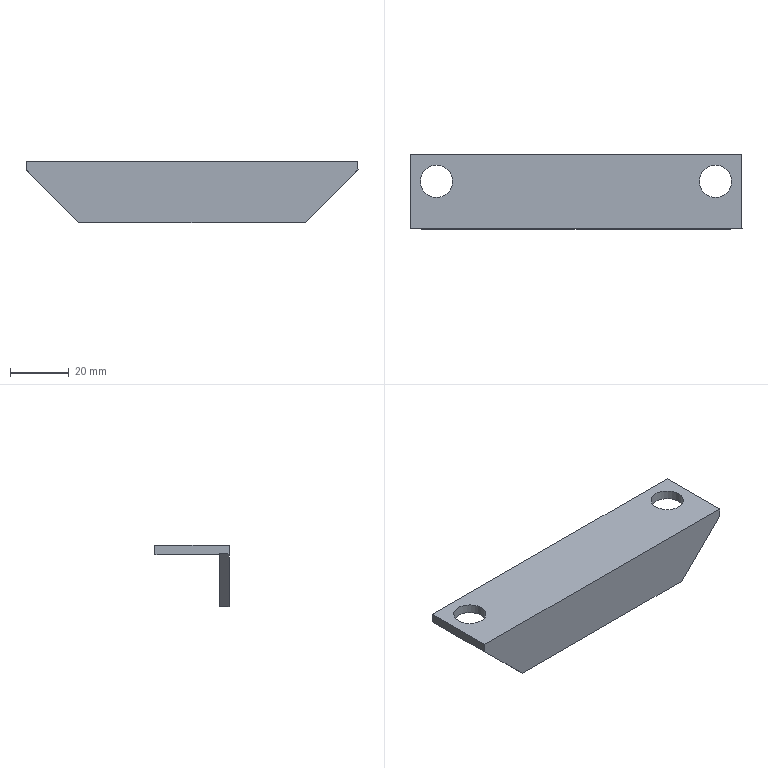Part | NX | features solid 2 | 1 solid | 14 faces | box 113 x 25.2 x 21 mm | volume 13904 mm3 | plane 12 | cylinder 2 | commonest cylinder face diameters 11 x2
STEP:
#1=CARTESIAN_POINT('',(-352.8,-53.5,401.8));
#2=VERTEX_POINT('',#1);
#3=CARTESIAN_POINT('',(-240.2,-53.5,401.8));
#4=VERTEX_POINT('',#3);
#5=CARTESIAN_POINT('',(-353.,-53.5,401.8));
#6=DIRECTION('',(1.,0.000000011,0.000000001));
#7=VECTOR('',#6,1000.);
#8=LINE('',#5,#7);
#9=EDGE_CURVE('',#2,#4,#8,.T.);
#10=ORIENTED_EDGE('',*,*,#9,.T.);
#11=CARTESIAN_POINT('',(-258.,-53.5,384.));
#12=VERTEX_POINT('',#11);
#13=CARTESIAN_POINT('',(-258.,-53.5,384.));
#14=DIRECTION('',(-0.7071,-0.000000128,-0.7071));
#15=VECTOR('',#14,1000.);
#16=LINE('',#13,#15);
#17=EDGE_CURVE('',#12,#4,#16,.F.);
#18=ORIENTED_EDGE('',*,*,#17,.F.);
#19=CARTESIAN_POINT('',(-335.,-53.5,384.));
#20=VERTEX_POINT('',#19);
#21=CARTESIAN_POINT('',(-353.,-53.5,384.));
#22=DIRECTION('',(1.,0.000000011,0.000000001));
#23=VECTOR('',#22,1000.);
#24=LINE('',#21,#23);
#25=EDGE_CURVE('',#20,#12,#24,.T.);
#26=ORIENTED_EDGE('',*,*,#25,.F.);
#27=CARTESIAN_POINT('',(-353.,-53.5,402.));
#28=DIRECTION('',(0.7071,-0.000000113,-0.7071));
#29=VECTOR('',#28,1000.);
#30=LINE('',#27,#29);
#31=EDGE_CURVE('',#2,#20,#30,.T.);
#32=ORIENTED_EDGE('',*,*,#31,.F.);
#33=EDGE_LOOP('',(#10,#18,#26,#32));
#34=FACE_BOUND('',#33,.T.);
#35=CARTESIAN_POINT('',(-353.,-53.5,379.));
#36=DIRECTION('',(0.000000011,-1.,0.00000017));
#37=DIRECTION('',(0.000000001,-0.00000017,-1.));
#38=AXIS2_PLACEMENT_3D('',#35,#36,#37);
#39=PLANE('',#38);
#40=ADVANCED_FACE('',(#34),#39,.F.);
#41=CARTESIAN_POINT('',(-353.,-56.7,405.));
#42=VERTEX_POINT('',#41);
#43=CARTESIAN_POINT('',(-240.,-56.7,405.));
#44=VERTEX_POINT('',#43);
#45=CARTESIAN_POINT('',(-353.,-56.7,405.));
#46=DIRECTION('',(1.,0.000000011,0.000000001));
#47=VECTOR('',#46,1000.);
#48=LINE('',#45,#47);
#49=EDGE_CURVE('',#42,#44,#48,.T.);
#50=ORIENTED_EDGE('',*,*,#49,.T.);
#51=CARTESIAN_POINT('',(-240.,-31.5,405.));
#52=VERTEX_POINT('',#51);
#53=CARTESIAN_POINT('',(-240.,-53.5,405.));
#54=DIRECTION('',(0.000000011,-1.,0.00000017));
#55=VECTOR('',#54,1000.);
#56=LINE('',#53,#55);
#57=EDGE_CURVE('',#52,#44,#56,.T.);
#58=ORIENTED_EDGE('',*,*,#57,.F.);
#59=CARTESIAN_POINT('',(-353.,-31.5,405.));
#60=VERTEX_POINT('',#59);
#61=CARTESIAN_POINT('',(-353.,-31.5,405.));
#62=DIRECTION('',(1.,0.000000011,0.000000001));
#63=VECTOR('',#62,1000.);
#64=LINE('',#61,#63);
#65=EDGE_CURVE('',#60,#52,#64,.T.);
#66=ORIENTED_EDGE('',*,*,#65,.F.);
#67=CARTESIAN_POINT('',(-353.,-53.5,405.));
#68=DIRECTION('',(0.000000011,-1.,0.00000017));
#69=VECTOR('',#68,1000.);
#70=LINE('',#67,#69);
#71=EDGE_CURVE('',#60,#42,#70,.T.);
#72=ORIENTED_EDGE('',*,*,#71,.T.);
#73=EDGE_LOOP('',(#50,#58,#66,#72));
#74=FACE_BOUND('',#73,.T.);
#75=CARTESIAN_POINT('',(-254.5,-40.5,405.));
#76=VERTEX_POINT('',#75);
#77=CARTESIAN_POINT('',(-249.,-40.5,405.));
#78=DIRECTION('',(-0.000000001,0.00000017,1.));
#79=DIRECTION('',(-1.,-0.000000011,-0.000000001));
#80=AXIS2_PLACEMENT_3D('',#77,#78,#79);
#81=CIRCLE('',#80,5.5);
#82=EDGE_CURVE('',#76,#76,#81,.F.);
#83=ORIENTED_EDGE('',*,*,#82,.T.);
#84=EDGE_LOOP('',(#83));
#85=FACE_BOUND('',#84,.T.);
#86=CARTESIAN_POINT('',(-349.5,-40.5,405.));
#87=VERTEX_POINT('',#86);
#88=CARTESIAN_POINT('',(-344.,-40.5,405.));
#89=DIRECTION('',(-0.000000001,0.00000017,1.));
#90=DIRECTION('',(-1.,-0.000000011,-0.000000001));
#91=AXIS2_PLACEMENT_3D('',#88,#89,#90);
#92=CIRCLE('',#91,5.5);
#93=EDGE_CURVE('',#87,#87,#92,.F.);
#94=ORIENTED_EDGE('',*,*,#93,.T.);
#95=EDGE_LOOP('',(#94));
#96=FACE_BOUND('',#95,.T.);
#97=CARTESIAN_POINT('',(-353.,-53.5,405.));
#98=DIRECTION('',(0.000000001,-0.00000017,-1.));
#99=DIRECTION('',(1.,0.000000011,0.000000001));
#100=AXIS2_PLACEMENT_3D('',#97,#98,#99);
#101=PLANE('',#100);
#102=ADVANCED_FACE('',(#74,#85,#96),#101,.F.);
#103=ORIENTED_EDGE('',*,*,#71,.F.);
#104=CARTESIAN_POINT('',(-353.,-31.5,401.8));
#105=VERTEX_POINT('',#104);
#106=CARTESIAN_POINT('',(-353.,-31.5,405.));
#107=DIRECTION('',(0.000000001,-0.00000017,-1.));
#108=VECTOR('',#107,1000.);
#109=LINE('',#106,#108);
#110=EDGE_CURVE('',#60,#105,#109,.T.);
#111=ORIENTED_EDGE('',*,*,#110,.T.);
#112=CARTESIAN_POINT('',(-353.,-53.5,401.8));
#113=VERTEX_POINT('',#112);
#114=CARTESIAN_POINT('',(-353.,-56.7,401.8));
#115=DIRECTION('',(0.000000011,-1.,0.00000017));
#116=VECTOR('',#115,1000.);
#117=LINE('',#114,#116);
#118=EDGE_CURVE('',#105,#113,#117,.T.);
#119=ORIENTED_EDGE('',*,*,#118,.T.);
#120=CARTESIAN_POINT('',(-353.,-53.5,402.));
#121=VERTEX_POINT('',#120);
#122=CARTESIAN_POINT('',(-353.,-53.5,405.));
#123=DIRECTION('',(0.000000001,-0.00000017,-1.));
#124=VECTOR('',#123,1000.);
#125=LINE('',#122,#124);
#126=EDGE_CURVE('',#121,#113,#125,.T.);
#127=ORIENTED_EDGE('',*,*,#126,.F.);
#128=CARTESIAN_POINT('',(-353.,-56.7,402.));
#129=VERTEX_POINT('',#128);
#130=CARTESIAN_POINT('',(-353.,-53.5,402.));
#131=DIRECTION('',(-0.000000011,1.,-0.00000017));
#132=VECTOR('',#131,1000.);
#133=LINE('',#130,#132);
#134=EDGE_CURVE('',#129,#121,#133,.T.);
#135=ORIENTED_EDGE('',*,*,#134,.F.);
#136=CARTESIAN_POINT('',(-353.,-56.7,405.));
#137=DIRECTION('',(0.000000001,-0.00000017,-1.));
#138=VECTOR('',#137,1000.);
#139=LINE('',#136,#138);
#140=EDGE_CURVE('',#42,#129,#139,.T.);
#141=ORIENTED_EDGE('',*,*,#140,.F.);
#142=EDGE_LOOP('',(#103,#111,#119,#127,#135,#141));
#143=FACE_BOUND('',#142,.T.);
#144=CARTESIAN_POINT('',(-353.,-53.5,405.));
#145=DIRECTION('',(-1.,-0.000000011,-0.000000001));
#146=DIRECTION('',(0.000000001,-0.00000017,-1.));
#147=AXIS2_PLACEMENT_3D('',#144,#145,#146);
#148=PLANE('',#147);
#149=ADVANCED_FACE('',(#143),#148,.T.);
#150=CARTESIAN_POINT('',(-240.,-56.7,402.));
#151=VERTEX_POINT('',#150);
#152=CARTESIAN_POINT('',(-240.,-56.7,405.));
#153=DIRECTION('',(0.000000001,-0.00000017,-1.));
#154=VECTOR('',#153,1000.);
#155=LINE('',#152,#154);
#156=EDGE_CURVE('',#44,#151,#155,.T.);
#157=ORIENTED_EDGE('',*,*,#156,.T.);
#158=CARTESIAN_POINT('',(-240.,-53.5,402.));
#159=VERTEX_POINT('',#158);
#160=CARTESIAN_POINT('',(-240.,-53.5,402.));
#161=DIRECTION('',(0.000000011,-1.,0.00000017));
#162=VECTOR('',#161,1000.);
#163=LINE('',#160,#162);
#164=EDGE_CURVE('',#159,#151,#163,.T.);
#165=ORIENTED_EDGE('',*,*,#164,.F.);
#166=CARTESIAN_POINT('',(-240.,-53.5,401.8));
#167=VERTEX_POINT('',#166);
#168=CARTESIAN_POINT('',(-240.,-53.5,405.));
#169=DIRECTION('',(0.000000001,-0.00000017,-1.));
#170=VECTOR('',#169,1000.);
#171=LINE('',#168,#170);
#172=EDGE_CURVE('',#159,#167,#171,.T.);
#173=ORIENTED_EDGE('',*,*,#172,.T.);
#174=CARTESIAN_POINT('',(-240.,-31.5,401.8));
#175=VERTEX_POINT('',#174);
#176=CARTESIAN_POINT('',(-240.,-56.7,401.8));
#177=DIRECTION('',(0.000000011,-1.,0.00000017));
#178=VECTOR('',#177,1000.);
#179=LINE('',#176,#178);
#180=EDGE_CURVE('',#175,#167,#179,.T.);
#181=ORIENTED_EDGE('',*,*,#180,.F.);
#182=CARTESIAN_POINT('',(-240.,-31.5,405.));
#183=DIRECTION('',(0.000000001,-0.00000017,-1.));
#184=VECTOR('',#183,1000.);
#185=LINE('',#182,#184);
#186=EDGE_CURVE('',#52,#175,#185,.T.);
#187=ORIENTED_EDGE('',*,*,#186,.F.);
#188=ORIENTED_EDGE('',*,*,#57,.T.);
#189=EDGE_LOOP('',(#157,#165,#173,#181,#187,#188));
#190=FACE_BOUND('',#189,.T.);
#191=CARTESIAN_POINT('',(-240.,-53.5,405.));
#192=DIRECTION('',(-1.,-0.000000011,-0.000000001));
#193=DIRECTION('',(0.000000001,-0.00000017,-1.));
#194=AXIS2_PLACEMENT_3D('',#191,#192,#193);
#195=PLANE('',#194);
#196=ADVANCED_FACE('',(#190),#195,.F.);
#197=CARTESIAN_POINT('',(-335.,-56.7,384.));
#198=VERTEX_POINT('',#197);
#199=CARTESIAN_POINT('',(-258.,-56.7,384.));
#200=VERTEX_POINT('',#199);
#201=CARTESIAN_POINT('',(-353.,-56.7,384.));
#202=DIRECTION('',(1.,0.000000011,0.000000001));
#203=VECTOR('',#202,1000.);
#204=LINE('',#201,#203);
#205=EDGE_CURVE('',#198,#200,#204,.T.);
#206=ORIENTED_EDGE('',*,*,#205,.T.);
#207=CARTESIAN_POINT('',(-258.,-56.7,384.));
#208=DIRECTION('',(0.7071,0.000000128,0.7071));
#209=VECTOR('',#208,1000.);
#210=LINE('',#207,#209);
#211=EDGE_CURVE('',#151,#200,#210,.F.);
#212=ORIENTED_EDGE('',*,*,#211,.F.);
#213=ORIENTED_EDGE('',*,*,#156,.F.);
#214=ORIENTED_EDGE('',*,*,#49,.F.);
#215=ORIENTED_EDGE('',*,*,#140,.T.);
#216=CARTESIAN_POINT('',(-353.,-56.7,402.));
#217=DIRECTION('',(-0.7071,0.000000113,0.7071));
#218=VECTOR('',#217,1000.);
#219=LINE('',#216,#218);
#220=EDGE_CURVE('',#198,#129,#219,.T.);
#221=ORIENTED_EDGE('',*,*,#220,.F.);
#222=EDGE_LOOP('',(#206,#212,#213,#214,#215,#221));
#223=FACE_BOUND('',#222,.T.);
#224=CARTESIAN_POINT('',(-353.,-56.7,402.));
#225=DIRECTION('',(-0.000000011,1.,-0.00000017));
#226=DIRECTION('',(-0.000000001,0.00000017,1.));
#227=AXIS2_PLACEMENT_3D('',#224,#225,#226);
#228=PLANE('',#227);
#229=ADVANCED_FACE('',(#223),#228,.F.);
#230=ORIENTED_EDGE('',*,*,#25,.T.);
#231=CARTESIAN_POINT('',(-258.,-56.7,384.));
#232=DIRECTION('',(-0.000000011,1.,-0.00000017));
#233=VECTOR('',#232,1000.);
#234=LINE('',#231,#233);
#235=EDGE_CURVE('',#200,#12,#234,.T.);
#236=ORIENTED_EDGE('',*,*,#235,.F.);
#237=ORIENTED_EDGE('',*,*,#205,.F.);
#238=CARTESIAN_POINT('',(-335.,-56.7,384.));
#239=DIRECTION('',(0.000000011,-1.,0.00000017));
#240=VECTOR('',#239,1000.);
#241=LINE('',#238,#240);
#242=EDGE_CURVE('',#20,#198,#241,.T.);
#243=ORIENTED_EDGE('',*,*,#242,.F.);
#244=EDGE_LOOP('',(#230,#236,#237,#243));
#245=FACE_BOUND('',#244,.T.);
#246=CARTESIAN_POINT('',(-353.,-56.7,384.));
#247=DIRECTION('',(-0.000000001,0.00000017,1.));
#248=DIRECTION('',(-1.,-0.000000011,-0.000000001));
#249=AXIS2_PLACEMENT_3D('',#246,#247,#248);
#250=PLANE('',#249);
#251=ADVANCED_FACE('',(#245),#250,.F.);
#252=ORIENTED_EDGE('',*,*,#220,.T.);
#253=ORIENTED_EDGE('',*,*,#134,.T.);
#254=CARTESIAN_POINT('',(-353.,-53.5,402.));
#255=DIRECTION('',(0.7071,-0.000000113,-0.7071));
#256=VECTOR('',#255,1000.);
#257=LINE('',#254,#256);
#258=EDGE_CURVE('',#121,#2,#257,.T.);
#259=ORIENTED_EDGE('',*,*,#258,.T.);
#260=ORIENTED_EDGE('',*,*,#31,.T.);
#261=ORIENTED_EDGE('',*,*,#242,.T.);
#262=EDGE_LOOP('',(#252,#253,#259,#260,#261));
#263=FACE_BOUND('',#262,.T.);
#264=CARTESIAN_POINT('',(-353.,-53.5,402.));
#265=DIRECTION('',(-0.7071,-0.000000128,-0.7071));
#266=DIRECTION('',(0.7071,-0.000000113,-0.7071));
#267=AXIS2_PLACEMENT_3D('',#264,#265,#266);
#268=PLANE('',#267);
#269=ADVANCED_FACE('',(#263),#268,.T.);
#270=ORIENTED_EDGE('',*,*,#211,.T.);
#271=ORIENTED_EDGE('',*,*,#235,.T.);
#272=ORIENTED_EDGE('',*,*,#17,.T.);
#273=CARTESIAN_POINT('',(-258.,-53.5,384.));
#274=DIRECTION('',(-0.7071,-0.000000128,-0.7071));
#275=VECTOR('',#274,1000.);
#276=LINE('',#273,#275);
#277=EDGE_CURVE('',#4,#159,#276,.F.);
#278=ORIENTED_EDGE('',*,*,#277,.T.);
#279=ORIENTED_EDGE('',*,*,#164,.T.);
#280=EDGE_LOOP('',(#270,#271,#272,#278,#279));
#281=FACE_BOUND('',#280,.T.);
#282=CARTESIAN_POINT('',(-258.,-56.7,384.));
#283=DIRECTION('',(-0.7071,0.000000113,0.7071));
#284=DIRECTION('',(-0.7071,-0.000000128,-0.7071));
#285=AXIS2_PLACEMENT_3D('',#282,#283,#284);
#286=PLANE('',#285);
#287=ADVANCED_FACE('',(#281),#286,.F.);
#288=ORIENTED_EDGE('',*,*,#126,.T.);
#289=CARTESIAN_POINT('',(-353.,-53.5,401.8));
#290=DIRECTION('',(1.,0.000000011,0.000000001));
#291=VECTOR('',#290,1000.);
#292=LINE('',#289,#291);
#293=EDGE_CURVE('',#113,#2,#292,.T.);
#294=ORIENTED_EDGE('',*,*,#293,.T.);
#295=ORIENTED_EDGE('',*,*,#258,.F.);
#296=EDGE_LOOP('',(#288,#294,#295));
#297=FACE_BOUND('',#296,.T.);
#298=CARTESIAN_POINT('',(-353.,-53.5,402.));
#299=DIRECTION('',(-0.000000011,1.,-0.00000017));
#300=DIRECTION('',(-0.000000001,0.00000017,1.));
#301=AXIS2_PLACEMENT_3D('',#298,#299,#300);
#302=PLANE('',#301);
#303=ADVANCED_FACE('',(#297),#302,.F.);
#304=CARTESIAN_POINT('',(-353.,-53.5,401.8));
#305=DIRECTION('',(1.,0.000000011,0.000000001));
#306=VECTOR('',#305,1000.);
#307=LINE('',#304,#306);
#308=EDGE_CURVE('',#4,#167,#307,.T.);
#309=ORIENTED_EDGE('',*,*,#308,.T.);
#310=ORIENTED_EDGE('',*,*,#172,.F.);
#311=ORIENTED_EDGE('',*,*,#277,.F.);
#312=EDGE_LOOP('',(#309,#310,#311));
#313=FACE_BOUND('',#312,.T.);
#314=CARTESIAN_POINT('',(-353.,-53.5,402.));
#315=DIRECTION('',(-0.000000011,1.,-0.00000017));
#316=DIRECTION('',(-0.000000001,0.00000017,1.));
#317=AXIS2_PLACEMENT_3D('',#314,#315,#316);
#318=PLANE('',#317);
#319=ADVANCED_FACE('',(#313),#318,.F.);
#320=CARTESIAN_POINT('',(-243.5,-40.5,401.8));
#321=VERTEX_POINT('',#320);
#322=CARTESIAN_POINT('',(-249.,-40.5,401.8));
#323=DIRECTION('',(-0.000000001,0.00000017,1.));
#324=DIRECTION('',(1.,0.000000011,0.000000001));
#325=AXIS2_PLACEMENT_3D('',#322,#323,#324);
#326=CIRCLE('',#325,5.5);
#327=EDGE_CURVE('',#321,#321,#326,.T.);
#328=ORIENTED_EDGE('',*,*,#327,.T.);
#329=EDGE_LOOP('',(#328));
#330=FACE_BOUND('',#329,.T.);
#331=ORIENTED_EDGE('',*,*,#180,.T.);
#332=ORIENTED_EDGE('',*,*,#308,.F.);
#333=ORIENTED_EDGE('',*,*,#9,.F.);
#334=ORIENTED_EDGE('',*,*,#293,.F.);
#335=ORIENTED_EDGE('',*,*,#118,.F.);
#336=CARTESIAN_POINT('',(-353.,-31.5,401.8));
#337=DIRECTION('',(1.,0.000000011,0.000000001));
#338=VECTOR('',#337,1000.);
#339=LINE('',#336,#338);
#340=EDGE_CURVE('',#105,#175,#339,.T.);
#341=ORIENTED_EDGE('',*,*,#340,.T.);
#342=EDGE_LOOP('',(#331,#332,#333,#334,#335,#341));
#343=FACE_BOUND('',#342,.T.);
#344=CARTESIAN_POINT('',(-349.5,-40.5,401.8));
#345=VERTEX_POINT('',#344);
#346=CARTESIAN_POINT('',(-344.,-40.5,401.8));
#347=DIRECTION('',(0.000000001,-0.00000017,-1.));
#348=DIRECTION('',(-1.,-0.000000011,-0.000000001));
#349=AXIS2_PLACEMENT_3D('',#346,#347,#348);
#350=CIRCLE('',#349,5.5);
#351=EDGE_CURVE('',#345,#345,#350,.T.);
#352=ORIENTED_EDGE('',*,*,#351,.F.);
#353=EDGE_LOOP('',(#352));
#354=FACE_BOUND('',#353,.T.);
#355=CARTESIAN_POINT('',(-353.,-31.5,401.8));
#356=DIRECTION('',(-0.000000001,0.00000017,1.));
#357=DIRECTION('',(-1.,-0.000000011,-0.000000001));
#358=AXIS2_PLACEMENT_3D('',#355,#356,#357);
#359=PLANE('',#358);
#360=ADVANCED_FACE('',(#330,#343,#354),#359,.F.);
#361=ORIENTED_EDGE('',*,*,#186,.T.);
#362=ORIENTED_EDGE('',*,*,#340,.F.);
#363=ORIENTED_EDGE('',*,*,#110,.F.);
#364=ORIENTED_EDGE('',*,*,#65,.T.);
#365=EDGE_LOOP('',(#361,#362,#363,#364));
#366=FACE_BOUND('',#365,.T.);
#367=CARTESIAN_POINT('',(-353.,-31.5,405.));
#368=DIRECTION('',(0.000000011,-1.,0.00000017));
#369=DIRECTION('',(-0.000000001,0.00000017,1.));
#370=AXIS2_PLACEMENT_3D('',#367,#368,#369);
#371=PLANE('',#370);
#372=ADVANCED_FACE('',(#366),#371,.F.);
#373=ORIENTED_EDGE('',*,*,#327,.F.);
#374=EDGE_LOOP('',(#373));
#375=FACE_BOUND('',#374,.T.);
#376=ORIENTED_EDGE('',*,*,#82,.F.);
#377=EDGE_LOOP('',(#376));
#378=FACE_BOUND('',#377,.T.);
#379=CARTESIAN_POINT('',(-249.,-40.5,401.8));
#380=DIRECTION('',(-0.000000001,0.00000017,1.));
#381=DIRECTION('',(-1.,-0.000000011,-0.000000001));
#382=AXIS2_PLACEMENT_3D('',#379,#380,#381);
#383=CYLINDRICAL_SURFACE('',#382,5.5);
#384=ADVANCED_FACE('',(#375,#378),#383,.F.);
#385=ORIENTED_EDGE('',*,*,#351,.T.);
#386=EDGE_LOOP('',(#385));
#387=FACE_BOUND('',#386,.T.);
#388=ORIENTED_EDGE('',*,*,#93,.F.);
#389=EDGE_LOOP('',(#388));
#390=FACE_BOUND('',#389,.T.);
#391=CARTESIAN_POINT('',(-344.,-40.5,401.8));
#392=DIRECTION('',(-0.000000001,0.00000017,1.));
#393=DIRECTION('',(1.,0.000000011,0.000000001));
#394=AXIS2_PLACEMENT_3D('',#391,#392,#393);
#395=CYLINDRICAL_SURFACE('',#394,5.5);
#396=ADVANCED_FACE('',(#387,#390),#395,.F.);
#397=CLOSED_SHELL('',(#40,#102,#149,#196,#229,#251,#269,#287,#303,#319,#360,#372,#384,#396));
#398=MANIFOLD_SOLID_BREP('',#397);
#399=(LENGTH_UNIT()NAMED_UNIT(*)SI_UNIT(.MILLI.,.METRE.));
#400=UNCERTAINTY_MEASURE_WITH_UNIT(LENGTH_MEASURE(0.00001),#399,'','');
#401=(NAMED_UNIT(*)PLANE_ANGLE_UNIT()SI_UNIT($,.RADIAN.));
#402=(NAMED_UNIT(*)SI_UNIT($,.STERADIAN.)SOLID_ANGLE_UNIT());
#403=(GEOMETRIC_REPRESENTATION_CONTEXT(3)GLOBAL_UNCERTAINTY_ASSIGNED_CONTEXT((#400))GLOBAL_UNIT_ASSIGNED_CONTEXT((#399,#401,#402))REPRESENTATION_CONTEXT('',''));
#404=ADVANCED_BREP_SHAPE_REPRESENTATION('',(#398),#403);